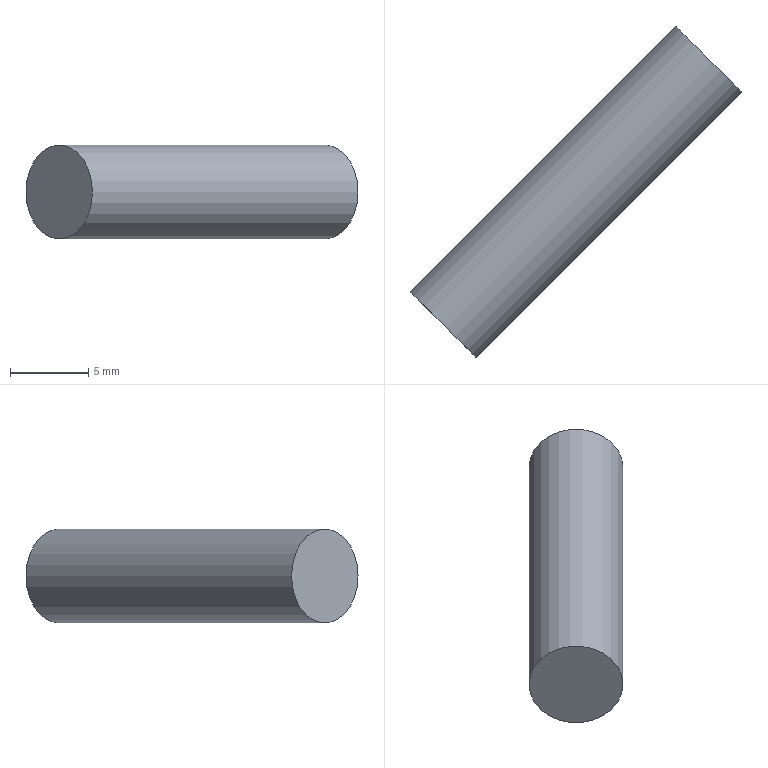Part | STEP file | gslz 2016.10.28-13_id658_x_t | 1 solid | 3 faces | box 21.213 x 21.213 x 6 mm | volume 678.584 mm3 | plane 2 | cylinder 1 | commonest cylinder face diameters 6 x1
STEP:
#1=CARTESIAN_POINT('',(0.,0.,0.));
#2=DIRECTION('',(0.,0.,1.));
#3=DIRECTION('',(1.,0.,0.));
#4=AXIS2_PLACEMENT_3D('',#1,#2,#3);
#5=CARTESIAN_POINT('',(578.491,186.956,-21.226));
#6=VERTEX_POINT('',#5);
#7=CARTESIAN_POINT('',(580.612,184.834,-21.226));
#8=DIRECTION('',(0.7071,0.7071,0.));
#9=DIRECTION('',(-0.7071,0.7071,0.));
#10=AXIS2_PLACEMENT_3D('',#7,#8,#9);
#11=CIRCLE('',#10,3.);
#12=CARTESIAN_POINT('',(580.612,184.834,-21.226));
#13=DIRECTION('',(-0.7071,-0.7071,0.));
#14=DIRECTION('',(0.7071,-0.7071,0.));
#15=AXIS2_PLACEMENT_3D('',#12,#13,#14);
#16=CYLINDRICAL_SURFACE('',#15,3.);
#17=CARTESIAN_POINT('',(9.425,0.));
#18=DIRECTION('',(-1.,0.));
#19=VECTOR('',#18,1.);
#20=LINE('',#17,#19);
#21=(GEOMETRIC_REPRESENTATION_CONTEXT(2)PARAMETRIC_REPRESENTATION_CONTEXT()REPRESENTATION_CONTEXT('',''));
#22=DEFINITIONAL_REPRESENTATION('',(#20),#21);
#23=PCURVE('',#16,#22);
#24=CARTESIAN_POINT('',(580.612,184.834,-21.226));
#25=DIRECTION('',(0.7071,0.7071,0.));
#26=DIRECTION('',(-0.7071,0.7071,0.));
#27=AXIS2_PLACEMENT_3D('',#24,#25,#26);
#28=PLANE('',#27);
#29=CARTESIAN_POINT('',(0.,0.));
#30=DIRECTION('',(1.,0.));
#31=AXIS2_PLACEMENT_2D('',#29,#30);
#32=CIRCLE('',#31,3.);
#33=(GEOMETRIC_REPRESENTATION_CONTEXT(2)PARAMETRIC_REPRESENTATION_CONTEXT()REPRESENTATION_CONTEXT('',''));
#34=DEFINITIONAL_REPRESENTATION('',(#32),#33);
#35=PCURVE('',#28,#34);
#36=SURFACE_CURVE('',#11,(#23,#35),.PCURVE_S1.);
#37=EDGE_CURVE('',#6,#6,#36,.T.);
#38=ORIENTED_EDGE('',*,*,#37,.F.);
#39=CARTESIAN_POINT('',(561.52,169.985,-21.226));
#40=VERTEX_POINT('',#39);
#41=CARTESIAN_POINT('',(578.491,186.956,-21.226));
#42=CARTESIAN_POINT('',(561.52,169.985,-21.226));
#43=B_SPLINE_CURVE_WITH_KNOTS('',1,(#41,#42),.UNSPECIFIED.,.F.,.F.,(2,2),(0.,24.),.PIECEWISE_BEZIER_KNOTS.);
#44=CARTESIAN_POINT('',(9.425,0.));
#45=DIRECTION('',(0.,1.));
#46=VECTOR('',#45,1.);
#47=LINE('',#44,#46);
#48=(GEOMETRIC_REPRESENTATION_CONTEXT(2)PARAMETRIC_REPRESENTATION_CONTEXT()REPRESENTATION_CONTEXT('',''));
#49=DEFINITIONAL_REPRESENTATION('',(#47),#48);
#50=PCURVE('',#16,#49);
#51=CARTESIAN_POINT('',(3.142,0.));
#52=DIRECTION('',(0.,1.));
#53=VECTOR('',#52,1.);
#54=LINE('',#51,#53);
#55=(GEOMETRIC_REPRESENTATION_CONTEXT(2)PARAMETRIC_REPRESENTATION_CONTEXT()REPRESENTATION_CONTEXT('',''));
#56=DEFINITIONAL_REPRESENTATION('',(#54),#55);
#57=PCURVE('',#16,#56);
#58=SEAM_CURVE('',#43,(#50,#57),.PCURVE_S1.);
#59=EDGE_CURVE('',#6,#40,#58,.T.);
#60=ORIENTED_EDGE('',*,*,#59,.T.);
#61=CARTESIAN_POINT('',(563.641,167.864,-21.226));
#62=DIRECTION('',(0.7071,0.7071,0.));
#63=DIRECTION('',(-0.7071,0.7071,0.));
#64=AXIS2_PLACEMENT_3D('',#61,#62,#63);
#65=CIRCLE('',#64,3.);
#66=CARTESIAN_POINT('',(9.425,24.));
#67=DIRECTION('',(-1.,0.));
#68=VECTOR('',#67,1.);
#69=LINE('',#66,#68);
#70=(GEOMETRIC_REPRESENTATION_CONTEXT(2)PARAMETRIC_REPRESENTATION_CONTEXT()REPRESENTATION_CONTEXT('',''));
#71=DEFINITIONAL_REPRESENTATION('',(#69),#70);
#72=PCURVE('',#16,#71);
#73=CARTESIAN_POINT('',(563.641,167.864,-21.226));
#74=DIRECTION('',(0.7071,0.7071,0.));
#75=DIRECTION('',(-0.7071,0.7071,0.));
#76=AXIS2_PLACEMENT_3D('',#73,#74,#75);
#77=PLANE('',#76);
#78=CARTESIAN_POINT('',(0.,0.));
#79=DIRECTION('',(1.,0.));
#80=AXIS2_PLACEMENT_2D('',#78,#79);
#81=CIRCLE('',#80,3.);
#82=(GEOMETRIC_REPRESENTATION_CONTEXT(2)PARAMETRIC_REPRESENTATION_CONTEXT()REPRESENTATION_CONTEXT('',''));
#83=DEFINITIONAL_REPRESENTATION('',(#81),#82);
#84=PCURVE('',#77,#83);
#85=SURFACE_CURVE('',#65,(#72,#84),.PCURVE_S1.);
#86=EDGE_CURVE('',#40,#40,#85,.T.);
#87=ORIENTED_EDGE('',*,*,#86,.T.);
#88=ORIENTED_EDGE('',*,*,#59,.F.);
#89=EDGE_LOOP('',(#38,#60,#87,#88));
#90=FACE_BOUND('',#89,.T.);
#91=ADVANCED_FACE('',(#90),#16,.T.);
#92=ORIENTED_EDGE('',*,*,#37,.T.);
#93=EDGE_LOOP('',(#92));
#94=FACE_BOUND('',#93,.T.);
#95=ADVANCED_FACE('',(#94),#28,.T.);
#96=ORIENTED_EDGE('',*,*,#86,.F.);
#97=EDGE_LOOP('',(#96));
#98=FACE_BOUND('',#97,.T.);
#99=ADVANCED_FACE('',(#98),#77,.F.);
#100=CLOSED_SHELL('',(#91,#95,#99));
#101=MANIFOLD_SOLID_BREP('',#100);
#102=(LENGTH_UNIT()NAMED_UNIT(*)SI_UNIT(.MILLI.,.METRE.));
#103=UNCERTAINTY_MEASURE_WITH_UNIT(LENGTH_MEASURE(0.00001),#102,'','');
#104=(NAMED_UNIT(*)PLANE_ANGLE_UNIT()SI_UNIT($,.RADIAN.));
#105=(NAMED_UNIT(*)SI_UNIT($,.STERADIAN.)SOLID_ANGLE_UNIT());
#106=(GEOMETRIC_REPRESENTATION_CONTEXT(3)GLOBAL_UNCERTAINTY_ASSIGNED_CONTEXT((#103))GLOBAL_UNIT_ASSIGNED_CONTEXT((#102,#104,#105))REPRESENTATION_CONTEXT('',''));
#107=ADVANCED_BREP_SHAPE_REPRESENTATION('',(#4,#101),#106);